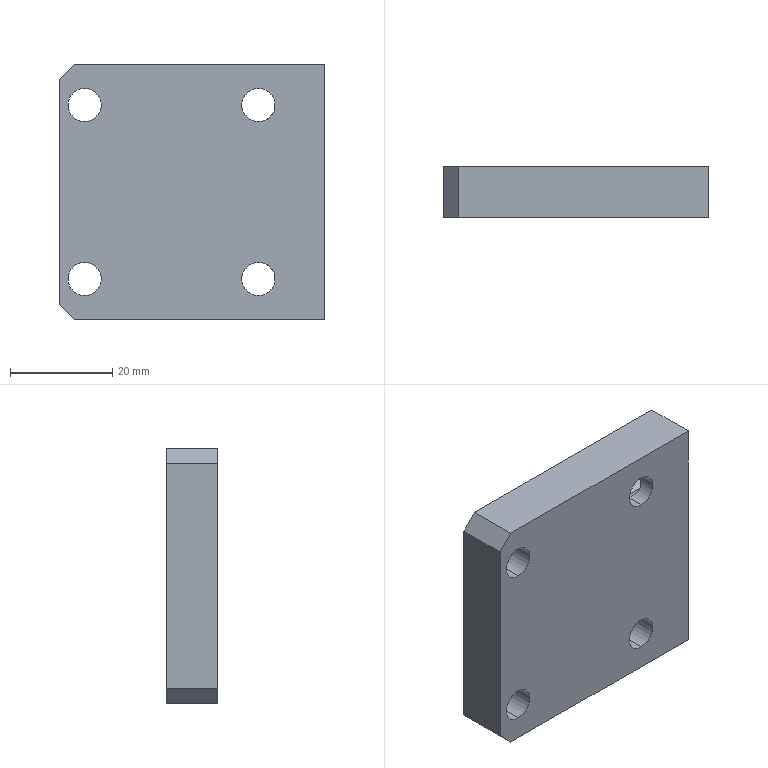Part | STEP file | PN_0010 | 1 solid | 39 faces | box 52 x 10 x 50 mm | volume 23516 mm3 | cylinder 20 | cone 11 | plane 8 | commonest cylinder face diameters 4.2 x8 6.5 x8 5 x4